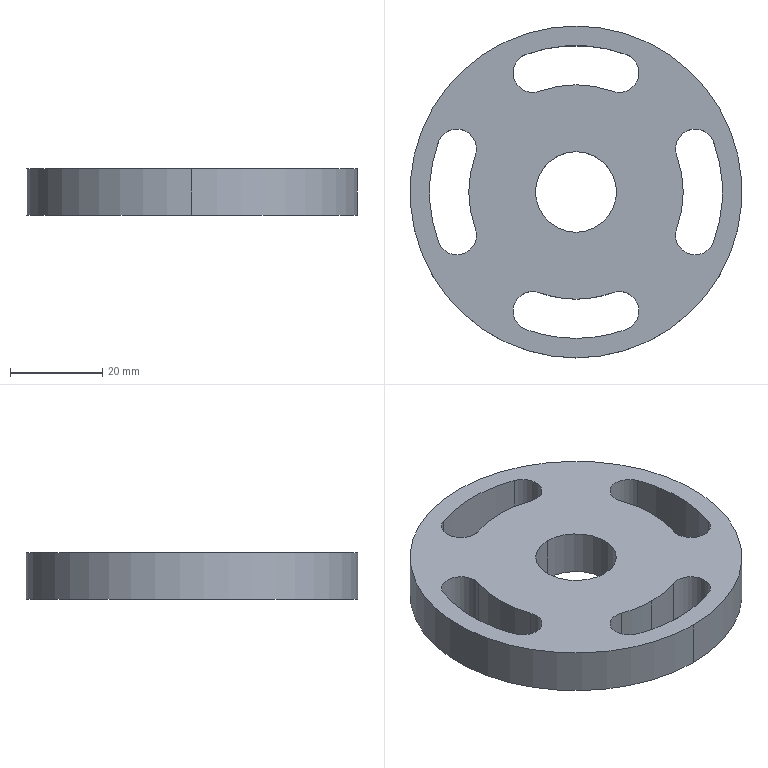Part | NX | 1 solid | 28 faces | box 72 x 72 x 10 mm | volume 29512 mm3 | cylinder 26 | plane 2 | commonest cylinder face diameters 8.5 x12 46.5 x5 63.5 x5 17.5 x2 72 x2
STEP:
#1=CARTESIAN_POINT('',(25.842,-13.656,0.));
#2=VERTEX_POINT('',#1);
#3=CARTESIAN_POINT('',(21.848,-7.952,0.));
#4=VERTEX_POINT('',#3);
#5=CARTESIAN_POINT('',(25.842,-9.406,0.));
#6=DIRECTION('',(0.,0.,-1.));
#7=DIRECTION('',(-1.,0.,0.));
#8=AXIS2_PLACEMENT_3D('',#5,#6,#7);
#9=CIRCLE('',#8,4.25);
#10=EDGE_CURVE('',#2,#4,#9,.T.);
#11=ORIENTED_EDGE('',*,*,#10,.F.);
#12=CARTESIAN_POINT('',(25.842,-13.656,-10.));
#13=VERTEX_POINT('',#12);
#14=CARTESIAN_POINT('',(25.842,-13.656,0.));
#15=DIRECTION('',(0.,0.,-1.));
#16=VECTOR('',#15,1000.);
#17=LINE('',#14,#16);
#18=EDGE_CURVE('',#2,#13,#17,.T.);
#19=ORIENTED_EDGE('',*,*,#18,.T.);
#20=CARTESIAN_POINT('',(21.848,-7.952,-10.));
#21=VERTEX_POINT('',#20);
#22=CARTESIAN_POINT('',(25.842,-9.406,-10.));
#23=DIRECTION('',(0.,0.,-1.));
#24=DIRECTION('',(-1.,0.,0.));
#25=AXIS2_PLACEMENT_3D('',#22,#23,#24);
#26=CIRCLE('',#25,4.25);
#27=EDGE_CURVE('',#13,#21,#26,.T.);
#28=ORIENTED_EDGE('',*,*,#27,.T.);
#29=CARTESIAN_POINT('',(21.848,-7.952,0.));
#30=DIRECTION('',(0.,0.,-1.));
#31=VECTOR('',#30,1000.);
#32=LINE('',#29,#31);
#33=EDGE_CURVE('',#4,#21,#32,.T.);
#34=ORIENTED_EDGE('',*,*,#33,.F.);
#35=EDGE_LOOP('',(#11,#19,#28,#34));
#36=FACE_BOUND('',#35,.T.);
#37=CARTESIAN_POINT('',(25.842,-9.406,0.));
#38=DIRECTION('',(0.,0.,-1.));
#39=DIRECTION('',(0.,1.,0.));
#40=AXIS2_PLACEMENT_3D('',#37,#38,#39);
#41=CYLINDRICAL_SURFACE('',#40,4.25);
#42=ADVANCED_FACE('',(#36),#41,.F.);
#43=CARTESIAN_POINT('',(0.,-31.75,0.));
#44=VERTEX_POINT('',#43);
#45=CARTESIAN_POINT('',(-10.859,-29.835,0.));
#46=VERTEX_POINT('',#45);
#47=CARTESIAN_POINT('',(0.,0.,0.));
#48=DIRECTION('',(0.,0.,-1.));
#49=DIRECTION('',(0.,1.,0.));
#50=AXIS2_PLACEMENT_3D('',#47,#48,#49);
#51=CIRCLE('',#50,31.75);
#52=EDGE_CURVE('',#44,#46,#51,.T.);
#53=ORIENTED_EDGE('',*,*,#52,.F.);
#54=CARTESIAN_POINT('',(0.,-31.75,-10.));
#55=VERTEX_POINT('',#54);
#56=CARTESIAN_POINT('',(0.,-31.75,0.));
#57=DIRECTION('',(0.,0.,-1.));
#58=VECTOR('',#57,1000.);
#59=LINE('',#56,#58);
#60=EDGE_CURVE('',#44,#55,#59,.T.);
#61=ORIENTED_EDGE('',*,*,#60,.T.);
#62=CARTESIAN_POINT('',(-10.859,-29.835,-10.));
#63=VERTEX_POINT('',#62);
#64=CARTESIAN_POINT('',(0.,0.,-10.));
#65=DIRECTION('',(0.,0.,-1.));
#66=DIRECTION('',(0.,1.,0.));
#67=AXIS2_PLACEMENT_3D('',#64,#65,#66);
#68=CIRCLE('',#67,31.75);
#69=EDGE_CURVE('',#55,#63,#68,.T.);
#70=ORIENTED_EDGE('',*,*,#69,.T.);
#71=CARTESIAN_POINT('',(-10.859,-29.835,0.));
#72=DIRECTION('',(0.,0.,-1.));
#73=VECTOR('',#72,1000.);
#74=LINE('',#71,#73);
#75=EDGE_CURVE('',#46,#63,#74,.T.);
#76=ORIENTED_EDGE('',*,*,#75,.F.);
#77=EDGE_LOOP('',(#53,#61,#70,#76));
#78=FACE_BOUND('',#77,.T.);
#79=CARTESIAN_POINT('',(0.,0.,0.));
#80=DIRECTION('',(0.,0.,-1.));
#81=DIRECTION('',(0.,1.,0.));
#82=AXIS2_PLACEMENT_3D('',#79,#80,#81);
#83=CYLINDRICAL_SURFACE('',#82,31.75);
#84=ADVANCED_FACE('',(#78),#83,.F.);
#85=CARTESIAN_POINT('',(0.,-23.25,0.));
#86=VERTEX_POINT('',#85);
#87=CARTESIAN_POINT('',(7.952,-21.848,0.));
#88=VERTEX_POINT('',#87);
#89=CARTESIAN_POINT('',(0.,0.,0.));
#90=DIRECTION('',(0.,0.,1.));
#91=DIRECTION('',(0.,1.,0.));
#92=AXIS2_PLACEMENT_3D('',#89,#90,#91);
#93=CIRCLE('',#92,23.25);
#94=EDGE_CURVE('',#86,#88,#93,.T.);
#95=ORIENTED_EDGE('',*,*,#94,.F.);
#96=CARTESIAN_POINT('',(0.,-23.25,-10.));
#97=VERTEX_POINT('',#96);
#98=CARTESIAN_POINT('',(0.,-23.25,0.));
#99=DIRECTION('',(0.,0.,-1.));
#100=VECTOR('',#99,1000.);
#101=LINE('',#98,#100);
#102=EDGE_CURVE('',#86,#97,#101,.T.);
#103=ORIENTED_EDGE('',*,*,#102,.T.);
#104=CARTESIAN_POINT('',(7.952,-21.848,-10.));
#105=VERTEX_POINT('',#104);
#106=CARTESIAN_POINT('',(0.,0.,-10.));
#107=DIRECTION('',(0.,0.,1.));
#108=DIRECTION('',(0.,1.,0.));
#109=AXIS2_PLACEMENT_3D('',#106,#107,#108);
#110=CIRCLE('',#109,23.25);
#111=EDGE_CURVE('',#97,#105,#110,.T.);
#112=ORIENTED_EDGE('',*,*,#111,.T.);
#113=CARTESIAN_POINT('',(7.952,-21.848,0.));
#114=DIRECTION('',(0.,0.,-1.));
#115=VECTOR('',#114,1000.);
#116=LINE('',#113,#115);
#117=EDGE_CURVE('',#88,#105,#116,.T.);
#118=ORIENTED_EDGE('',*,*,#117,.F.);
#119=EDGE_LOOP('',(#95,#103,#112,#118));
#120=FACE_BOUND('',#119,.T.);
#121=CARTESIAN_POINT('',(0.,0.,0.));
#122=DIRECTION('',(0.,0.,-1.));
#123=DIRECTION('',(0.,1.,0.));
#124=AXIS2_PLACEMENT_3D('',#121,#122,#123);
#125=CYLINDRICAL_SURFACE('',#124,23.25);
#126=ADVANCED_FACE('',(#120),#125,.T.);
#127=CARTESIAN_POINT('',(-25.842,-13.656,0.));
#128=VERTEX_POINT('',#127);
#129=CARTESIAN_POINT('',(-29.835,-10.859,0.));
#130=VERTEX_POINT('',#129);
#131=CARTESIAN_POINT('',(-25.842,-9.406,0.));
#132=DIRECTION('',(0.,0.,-1.));
#133=DIRECTION('',(1.,0.,0.));
#134=AXIS2_PLACEMENT_3D('',#131,#132,#133);
#135=CIRCLE('',#134,4.25);
#136=EDGE_CURVE('',#128,#130,#135,.T.);
#137=ORIENTED_EDGE('',*,*,#136,.F.);
#138=CARTESIAN_POINT('',(-25.842,-13.656,-10.));
#139=VERTEX_POINT('',#138);
#140=CARTESIAN_POINT('',(-25.842,-13.656,0.));
#141=DIRECTION('',(0.,0.,-1.));
#142=VECTOR('',#141,1000.);
#143=LINE('',#140,#142);
#144=EDGE_CURVE('',#128,#139,#143,.T.);
#145=ORIENTED_EDGE('',*,*,#144,.T.);
#146=CARTESIAN_POINT('',(-29.835,-10.859,-10.));
#147=VERTEX_POINT('',#146);
#148=CARTESIAN_POINT('',(-25.842,-9.406,-10.));
#149=DIRECTION('',(0.,0.,-1.));
#150=DIRECTION('',(1.,0.,0.));
#151=AXIS2_PLACEMENT_3D('',#148,#149,#150);
#152=CIRCLE('',#151,4.25);
#153=EDGE_CURVE('',#139,#147,#152,.T.);
#154=ORIENTED_EDGE('',*,*,#153,.T.);
#155=CARTESIAN_POINT('',(-29.835,-10.859,0.));
#156=DIRECTION('',(0.,0.,-1.));
#157=VECTOR('',#156,1000.);
#158=LINE('',#155,#157);
#159=EDGE_CURVE('',#130,#147,#158,.T.);
#160=ORIENTED_EDGE('',*,*,#159,.F.);
#161=EDGE_LOOP('',(#137,#145,#154,#160));
#162=FACE_BOUND('',#161,.T.);
#163=CARTESIAN_POINT('',(-25.842,-9.406,0.));
#164=DIRECTION('',(0.,0.,-1.));
#165=DIRECTION('',(0.,1.,0.));
#166=AXIS2_PLACEMENT_3D('',#163,#164,#165);
#167=CYLINDRICAL_SURFACE('',#166,4.25);
#168=ADVANCED_FACE('',(#162),#167,.F.);
#169=CARTESIAN_POINT('',(9.406,21.592,0.));
#170=VERTEX_POINT('',#169);
#171=CARTESIAN_POINT('',(7.952,21.848,0.));
#172=VERTEX_POINT('',#171);
#173=CARTESIAN_POINT('',(9.406,25.842,0.));
#174=DIRECTION('',(0.,0.,-1.));
#175=DIRECTION('',(0.,-1.,0.));
#176=AXIS2_PLACEMENT_3D('',#173,#174,#175);
#177=CIRCLE('',#176,4.25);
#178=EDGE_CURVE('',#170,#172,#177,.T.);
#179=ORIENTED_EDGE('',*,*,#178,.F.);
#180=CARTESIAN_POINT('',(9.406,21.592,-10.));
#181=VERTEX_POINT('',#180);
#182=CARTESIAN_POINT('',(9.406,21.592,0.));
#183=DIRECTION('',(0.,0.,-1.));
#184=VECTOR('',#183,1000.);
#185=LINE('',#182,#184);
#186=EDGE_CURVE('',#170,#181,#185,.T.);
#187=ORIENTED_EDGE('',*,*,#186,.T.);
#188=CARTESIAN_POINT('',(7.952,21.848,-10.));
#189=VERTEX_POINT('',#188);
#190=CARTESIAN_POINT('',(9.406,25.842,-10.));
#191=DIRECTION('',(0.,0.,-1.));
#192=DIRECTION('',(0.,-1.,0.));
#193=AXIS2_PLACEMENT_3D('',#190,#191,#192);
#194=CIRCLE('',#193,4.25);
#195=EDGE_CURVE('',#181,#189,#194,.T.);
#196=ORIENTED_EDGE('',*,*,#195,.T.);
#197=CARTESIAN_POINT('',(7.952,21.848,0.));
#198=DIRECTION('',(0.,0.,-1.));
#199=VECTOR('',#198,1000.);
#200=LINE('',#197,#199);
#201=EDGE_CURVE('',#172,#189,#200,.T.);
#202=ORIENTED_EDGE('',*,*,#201,.F.);
#203=EDGE_LOOP('',(#179,#187,#196,#202));
#204=FACE_BOUND('',#203,.T.);
#205=CARTESIAN_POINT('',(9.406,25.842,0.));
#206=DIRECTION('',(0.,0.,-1.));
#207=DIRECTION('',(0.,1.,0.));
#208=AXIS2_PLACEMENT_3D('',#205,#206,#207);
#209=CYLINDRICAL_SURFACE('',#208,4.25);
#210=ADVANCED_FACE('',(#204),#209,.F.);
#211=CARTESIAN_POINT('',(-9.406,21.592,0.));
#212=VERTEX_POINT('',#211);
#213=CARTESIAN_POINT('',(-10.859,29.835,0.));
#214=VERTEX_POINT('',#213);
#215=CARTESIAN_POINT('',(-9.406,25.842,0.));
#216=DIRECTION('',(0.,0.,-1.));
#217=DIRECTION('',(0.,-1.,0.));
#218=AXIS2_PLACEMENT_3D('',#215,#216,#217);
#219=CIRCLE('',#218,4.25);
#220=EDGE_CURVE('',#212,#214,#219,.T.);
#221=ORIENTED_EDGE('',*,*,#220,.F.);
#222=CARTESIAN_POINT('',(-9.406,21.592,-10.));
#223=VERTEX_POINT('',#222);
#224=CARTESIAN_POINT('',(-9.406,21.592,0.));
#225=DIRECTION('',(0.,0.,-1.));
#226=VECTOR('',#225,1000.);
#227=LINE('',#224,#226);
#228=EDGE_CURVE('',#212,#223,#227,.T.);
#229=ORIENTED_EDGE('',*,*,#228,.T.);
#230=CARTESIAN_POINT('',(-10.859,29.835,-10.));
#231=VERTEX_POINT('',#230);
#232=CARTESIAN_POINT('',(-9.406,25.842,-10.));
#233=DIRECTION('',(0.,0.,-1.));
#234=DIRECTION('',(0.,-1.,0.));
#235=AXIS2_PLACEMENT_3D('',#232,#233,#234);
#236=CIRCLE('',#235,4.25);
#237=EDGE_CURVE('',#223,#231,#236,.T.);
#238=ORIENTED_EDGE('',*,*,#237,.T.);
#239=CARTESIAN_POINT('',(-10.859,29.835,0.));
#240=DIRECTION('',(0.,0.,-1.));
#241=VECTOR('',#240,1000.);
#242=LINE('',#239,#241);
#243=EDGE_CURVE('',#214,#231,#242,.T.);
#244=ORIENTED_EDGE('',*,*,#243,.F.);
#245=EDGE_LOOP('',(#221,#229,#238,#244));
#246=FACE_BOUND('',#245,.T.);
#247=CARTESIAN_POINT('',(-9.406,25.842,0.));
#248=DIRECTION('',(0.,0.,-1.));
#249=DIRECTION('',(0.,1.,0.));
#250=AXIS2_PLACEMENT_3D('',#247,#248,#249);
#251=CYLINDRICAL_SURFACE('',#250,4.25);
#252=ADVANCED_FACE('',(#246),#251,.F.);
#253=CARTESIAN_POINT('',(0.,8.75,0.));
#254=VERTEX_POINT('',#253);
#255=CARTESIAN_POINT('',(0.,-8.75,0.));
#256=VERTEX_POINT('',#255);
#257=CARTESIAN_POINT('',(0.,0.,0.));
#258=DIRECTION('',(0.,0.,-1.));
#259=DIRECTION('',(0.,-1.,0.));
#260=AXIS2_PLACEMENT_3D('',#257,#258,#259);
#261=CIRCLE('',#260,8.75);
#262=EDGE_CURVE('',#254,#256,#261,.T.);
#263=ORIENTED_EDGE('',*,*,#262,.F.);
#264=CARTESIAN_POINT('',(0.,8.75,-10.));
#265=VERTEX_POINT('',#264);
#266=CARTESIAN_POINT('',(0.,8.75,-10.));
#267=DIRECTION('',(0.,0.,-1.));
#268=VECTOR('',#267,1000.);
#269=LINE('',#266,#268);
#270=EDGE_CURVE('',#265,#254,#269,.F.);
#271=ORIENTED_EDGE('',*,*,#270,.F.);
#272=CARTESIAN_POINT('',(0.,-8.75,-10.));
#273=VERTEX_POINT('',#272);
#274=CARTESIAN_POINT('',(0.,0.,-10.));
#275=DIRECTION('',(0.,0.,-1.));
#276=DIRECTION('',(0.,-1.,0.));
#277=AXIS2_PLACEMENT_3D('',#274,#275,#276);
#278=CIRCLE('',#277,8.75);
#279=EDGE_CURVE('',#265,#273,#278,.T.);
#280=ORIENTED_EDGE('',*,*,#279,.T.);
#281=CARTESIAN_POINT('',(0.,-8.75,-10.));
#282=DIRECTION('',(0.,0.,-1.));
#283=VECTOR('',#282,1000.);
#284=LINE('',#281,#283);
#285=EDGE_CURVE('',#273,#256,#284,.F.);
#286=ORIENTED_EDGE('',*,*,#285,.T.);
#287=EDGE_LOOP('',(#263,#271,#280,#286));
#288=FACE_BOUND('',#287,.T.);
#289=CARTESIAN_POINT('',(0.,0.,-10.));
#290=DIRECTION('',(0.,0.,-1.));
#291=DIRECTION('',(0.,1.,0.));
#292=AXIS2_PLACEMENT_3D('',#289,#290,#291);
#293=CYLINDRICAL_SURFACE('',#292,8.75);
#294=ADVANCED_FACE('',(#288),#293,.F.);
#295=CARTESIAN_POINT('',(0.,-36.,-10.));
#296=VERTEX_POINT('',#295);
#297=CARTESIAN_POINT('',(0.,36.,-10.));
#298=VERTEX_POINT('',#297);
#299=CARTESIAN_POINT('',(0.,0.,-10.));
#300=DIRECTION('',(0.,0.,-1.));
#301=DIRECTION('',(0.,-1.,0.));
#302=AXIS2_PLACEMENT_3D('',#299,#300,#301);
#303=CIRCLE('',#302,36.);
#304=EDGE_CURVE('',#296,#298,#303,.T.);
#305=ORIENTED_EDGE('',*,*,#304,.F.);
#306=CARTESIAN_POINT('',(0.,-36.,0.));
#307=VERTEX_POINT('',#306);
#308=CARTESIAN_POINT('',(0.,-36.,-10.));
#309=DIRECTION('',(0.,0.,1.));
#310=VECTOR('',#309,1000.);
#311=LINE('',#308,#310);
#312=EDGE_CURVE('',#307,#296,#311,.F.);
#313=ORIENTED_EDGE('',*,*,#312,.F.);
#314=CARTESIAN_POINT('',(0.,36.,0.));
#315=VERTEX_POINT('',#314);
#316=CARTESIAN_POINT('',(0.,0.,0.));
#317=DIRECTION('',(0.,0.,-1.));
#318=DIRECTION('',(0.,-1.,0.));
#319=AXIS2_PLACEMENT_3D('',#316,#317,#318);
#320=CIRCLE('',#319,36.);
#321=EDGE_CURVE('',#307,#315,#320,.T.);
#322=ORIENTED_EDGE('',*,*,#321,.T.);
#323=CARTESIAN_POINT('',(0.,36.,-10.));
#324=DIRECTION('',(0.,0.,1.));
#325=VECTOR('',#324,1000.);
#326=LINE('',#323,#325);
#327=EDGE_CURVE('',#315,#298,#326,.F.);
#328=ORIENTED_EDGE('',*,*,#327,.T.);
#329=EDGE_LOOP('',(#305,#313,#322,#328));
#330=FACE_BOUND('',#329,.T.);
#331=CARTESIAN_POINT('',(0.,0.,-10.));
#332=DIRECTION('',(0.,0.,1.));
#333=DIRECTION('',(0.,-1.,0.));
#334=AXIS2_PLACEMENT_3D('',#331,#332,#333);
#335=CYLINDRICAL_SURFACE('',#334,36.);
#336=ADVANCED_FACE('',(#330),#335,.T.);
#337=ORIENTED_EDGE('',*,*,#312,.T.);
#338=CARTESIAN_POINT('',(0.,0.,-10.));
#339=DIRECTION('',(0.,0.,-1.));
#340=DIRECTION('',(0.,-1.,0.));
#341=AXIS2_PLACEMENT_3D('',#338,#339,#340);
#342=CIRCLE('',#341,36.);
#343=EDGE_CURVE('',#298,#296,#342,.T.);
#344=ORIENTED_EDGE('',*,*,#343,.F.);
#345=ORIENTED_EDGE('',*,*,#327,.F.);
#346=CARTESIAN_POINT('',(0.,0.,0.));
#347=DIRECTION('',(0.,0.,-1.));
#348=DIRECTION('',(0.,-1.,0.));
#349=AXIS2_PLACEMENT_3D('',#346,#347,#348);
#350=CIRCLE('',#349,36.);
#351=EDGE_CURVE('',#315,#307,#350,.T.);
#352=ORIENTED_EDGE('',*,*,#351,.T.);
#353=EDGE_LOOP('',(#337,#344,#345,#352));
#354=FACE_BOUND('',#353,.T.);
#355=CARTESIAN_POINT('',(0.,0.,-10.));
#356=DIRECTION('',(0.,0.,1.));
#357=DIRECTION('',(0.,-1.,0.));
#358=AXIS2_PLACEMENT_3D('',#355,#356,#357);
#359=CYLINDRICAL_SURFACE('',#358,36.);
#360=ADVANCED_FACE('',(#354),#359,.T.);
#361=CARTESIAN_POINT('',(21.848,7.952,-10.));
#362=VERTEX_POINT('',#361);
#363=CARTESIAN_POINT('',(29.835,10.859,-10.));
#364=VERTEX_POINT('',#363);
#365=CARTESIAN_POINT('',(25.842,9.406,-10.));
#366=DIRECTION('',(0.,0.,-1.));
#367=DIRECTION('',(-1.,0.,0.));
#368=AXIS2_PLACEMENT_3D('',#365,#366,#367);
#369=CIRCLE('',#368,4.25);
#370=EDGE_CURVE('',#362,#364,#369,.T.);
#371=ORIENTED_EDGE('',*,*,#370,.F.);
#372=CARTESIAN_POINT('',(0.,0.,-10.));
#373=DIRECTION('',(0.,0.,1.));
#374=DIRECTION('',(-1.,0.,0.));
#375=AXIS2_PLACEMENT_3D('',#372,#373,#374);
#376=CIRCLE('',#375,23.25);
#377=EDGE_CURVE('',#21,#362,#376,.T.);
#378=ORIENTED_EDGE('',*,*,#377,.F.);
#379=ORIENTED_EDGE('',*,*,#27,.F.);
#380=CARTESIAN_POINT('',(29.835,-10.859,-10.));
#381=VERTEX_POINT('',#380);
#382=CARTESIAN_POINT('',(25.842,-9.406,-10.));
#383=DIRECTION('',(0.,0.,-1.));
#384=DIRECTION('',(-1.,0.,0.));
#385=AXIS2_PLACEMENT_3D('',#382,#383,#384);
#386=CIRCLE('',#385,4.25);
#387=EDGE_CURVE('',#381,#13,#386,.T.);
#388=ORIENTED_EDGE('',*,*,#387,.F.);
#389=CARTESIAN_POINT('',(0.,0.,-10.));
#390=DIRECTION('',(0.,0.,-1.));
#391=DIRECTION('',(-1.,0.,0.));
#392=AXIS2_PLACEMENT_3D('',#389,#390,#391);
#393=CIRCLE('',#392,31.75);
#394=EDGE_CURVE('',#364,#381,#393,.T.);
#395=ORIENTED_EDGE('',*,*,#394,.F.);
#396=EDGE_LOOP('',(#371,#378,#379,#388,#395));
#397=FACE_BOUND('',#396,.T.);
#398=CARTESIAN_POINT('',(10.859,-29.835,-10.));
#399=VERTEX_POINT('',#398);
#400=CARTESIAN_POINT('',(9.406,-25.842,-10.));
#401=DIRECTION('',(0.,0.,-1.));
#402=DIRECTION('',(0.,1.,0.));
#403=AXIS2_PLACEMENT_3D('',#400,#401,#402);
#404=CIRCLE('',#403,4.25);
#405=EDGE_CURVE('',#105,#399,#404,.T.);
#406=ORIENTED_EDGE('',*,*,#405,.F.);
#407=ORIENTED_EDGE('',*,*,#111,.F.);
#408=CARTESIAN_POINT('',(-7.952,-21.848,-10.));
#409=VERTEX_POINT('',#408);
#410=CARTESIAN_POINT('',(0.,0.,-10.));
#411=DIRECTION('',(0.,0.,1.));
#412=DIRECTION('',(0.,1.,0.));
#413=AXIS2_PLACEMENT_3D('',#410,#411,#412);
#414=CIRCLE('',#413,23.25);
#415=EDGE_CURVE('',#409,#97,#414,.T.);
#416=ORIENTED_EDGE('',*,*,#415,.F.);
#417=CARTESIAN_POINT('',(-9.406,-25.842,-10.));
#418=DIRECTION('',(0.,0.,-1.));
#419=DIRECTION('',(0.,1.,0.));
#420=AXIS2_PLACEMENT_3D('',#417,#418,#419);
#421=CIRCLE('',#420,4.25);
#422=EDGE_CURVE('',#63,#409,#421,.T.);
#423=ORIENTED_EDGE('',*,*,#422,.F.);
#424=ORIENTED_EDGE('',*,*,#69,.F.);
#425=CARTESIAN_POINT('',(0.,0.,-10.));
#426=DIRECTION('',(0.,0.,-1.));
#427=DIRECTION('',(0.,1.,0.));
#428=AXIS2_PLACEMENT_3D('',#425,#426,#427);
#429=CIRCLE('',#428,31.75);
#430=EDGE_CURVE('',#399,#55,#429,.T.);
#431=ORIENTED_EDGE('',*,*,#430,.F.);
#432=EDGE_LOOP('',(#406,#407,#416,#423,#424,#431));
#433=FACE_BOUND('',#432,.T.);
#434=CARTESIAN_POINT('',(-21.848,-7.952,-10.));
#435=VERTEX_POINT('',#434);
#436=CARTESIAN_POINT('',(-25.842,-9.406,-10.));
#437=DIRECTION('',(0.,0.,-1.));
#438=DIRECTION('',(1.,0.,0.));
#439=AXIS2_PLACEMENT_3D('',#436,#437,#438);
#440=CIRCLE('',#439,4.25);
#441=EDGE_CURVE('',#435,#139,#440,.T.);
#442=ORIENTED_EDGE('',*,*,#441,.F.);
#443=CARTESIAN_POINT('',(-21.848,7.952,-10.));
#444=VERTEX_POINT('',#443);
#445=CARTESIAN_POINT('',(0.,0.,-10.));
#446=DIRECTION('',(0.,0.,1.));
#447=DIRECTION('',(1.,0.,0.));
#448=AXIS2_PLACEMENT_3D('',#445,#446,#447);
#449=CIRCLE('',#448,23.25);
#450=EDGE_CURVE('',#444,#435,#449,.T.);
#451=ORIENTED_EDGE('',*,*,#450,.F.);
#452=CARTESIAN_POINT('',(-29.835,10.859,-10.));
#453=VERTEX_POINT('',#452);
#454=CARTESIAN_POINT('',(-25.842,9.406,-10.));
#455=DIRECTION('',(0.,0.,-1.));
#456=DIRECTION('',(1.,0.,0.));
#457=AXIS2_PLACEMENT_3D('',#454,#455,#456);
#458=CIRCLE('',#457,4.25);
#459=EDGE_CURVE('',#453,#444,#458,.T.);
#460=ORIENTED_EDGE('',*,*,#459,.F.);
#461=CARTESIAN_POINT('',(0.,0.,-10.));
#462=DIRECTION('',(0.,0.,-1.));
#463=DIRECTION('',(1.,0.,0.));
#464=AXIS2_PLACEMENT_3D('',#461,#462,#463);
#465=CIRCLE('',#464,31.75);
#466=EDGE_CURVE('',#147,#453,#465,.T.);
#467=ORIENTED_EDGE('',*,*,#466,.F.);
#468=ORIENTED_EDGE('',*,*,#153,.F.);
#469=EDGE_LOOP('',(#442,#451,#460,#467,#468));
#470=FACE_BOUND('',#469,.T.);
#471=CARTESIAN_POINT('',(-7.952,21.848,-10.));
#472=VERTEX_POINT('',#471);
#473=CARTESIAN_POINT('',(-9.406,25.842,-10.));
#474=DIRECTION('',(0.,0.,-1.));
#475=DIRECTION('',(0.,-1.,0.));
#476=AXIS2_PLACEMENT_3D('',#473,#474,#475);
#477=CIRCLE('',#476,4.25);
#478=EDGE_CURVE('',#472,#223,#477,.T.);
#479=ORIENTED_EDGE('',*,*,#478,.F.);
#480=CARTESIAN_POINT('',(0.,0.,-10.));
#481=DIRECTION('',(0.,0.,1.));
#482=DIRECTION('',(0.,-1.,0.));
#483=AXIS2_PLACEMENT_3D('',#480,#481,#482);
#484=CIRCLE('',#483,23.25);
#485=EDGE_CURVE('',#189,#472,#484,.T.);
#486=ORIENTED_EDGE('',*,*,#485,.F.);
#487=ORIENTED_EDGE('',*,*,#195,.F.);
#488=CARTESIAN_POINT('',(10.859,29.835,-10.));
#489=VERTEX_POINT('',#488);
#490=CARTESIAN_POINT('',(9.406,25.842,-10.));
#491=DIRECTION('',(0.,0.,-1.));
#492=DIRECTION('',(0.,-1.,0.));
#493=AXIS2_PLACEMENT_3D('',#490,#491,#492);
#494=CIRCLE('',#493,4.25);
#495=EDGE_CURVE('',#489,#181,#494,.T.);
#496=ORIENTED_EDGE('',*,*,#495,.F.);
#497=CARTESIAN_POINT('',(0.,0.,-10.));
#498=DIRECTION('',(0.,0.,-1.));
#499=DIRECTION('',(0.,-1.,0.));
#500=AXIS2_PLACEMENT_3D('',#497,#498,#499);
#501=CIRCLE('',#500,31.75);
#502=EDGE_CURVE('',#231,#489,#501,.T.);
#503=ORIENTED_EDGE('',*,*,#502,.F.);
#504=ORIENTED_EDGE('',*,*,#237,.F.);
#505=EDGE_LOOP('',(#479,#486,#487,#496,#503,#504));
#506=FACE_BOUND('',#505,.T.);
#507=CARTESIAN_POINT('',(0.,0.,-10.));
#508=DIRECTION('',(0.,0.,-1.));
#509=DIRECTION('',(0.,-1.,0.));
#510=AXIS2_PLACEMENT_3D('',#507,#508,#509);
#511=CIRCLE('',#510,8.75);
#512=EDGE_CURVE('',#273,#265,#511,.T.);
#513=ORIENTED_EDGE('',*,*,#512,.F.);
#514=ORIENTED_EDGE('',*,*,#279,.F.);
#515=EDGE_LOOP('',(#513,#514));
#516=FACE_BOUND('',#515,.T.);
#517=ORIENTED_EDGE('',*,*,#343,.T.);
#518=ORIENTED_EDGE('',*,*,#304,.T.);
#519=EDGE_LOOP('',(#517,#518));
#520=FACE_BOUND('',#519,.T.);
#521=CARTESIAN_POINT('',(0.,0.,-10.));
#522=DIRECTION('',(0.,0.,-1.));
#523=DIRECTION('',(0.,1.,0.));
#524=AXIS2_PLACEMENT_3D('',#521,#522,#523);
#525=PLANE('',#524);
#526=ADVANCED_FACE('',(#397,#433,#470,#506,#516,#520),#525,.T.);
#527=CARTESIAN_POINT('',(21.848,7.952,0.));
#528=VERTEX_POINT('',#527);
#529=CARTESIAN_POINT('',(0.,0.,0.));
#530=DIRECTION('',(0.,0.,1.));
#531=DIRECTION('',(-1.,0.,0.));
#532=AXIS2_PLACEMENT_3D('',#529,#530,#531);
#533=CIRCLE('',#532,23.25);
#534=EDGE_CURVE('',#4,#528,#533,.T.);
#535=ORIENTED_EDGE('',*,*,#534,.T.);
#536=CARTESIAN_POINT('',(29.835,10.859,0.));
#537=VERTEX_POINT('',#536);
#538=CARTESIAN_POINT('',(25.842,9.406,0.));
#539=DIRECTION('',(0.,0.,-1.));
#540=DIRECTION('',(-1.,0.,0.));
#541=AXIS2_PLACEMENT_3D('',#538,#539,#540);
#542=CIRCLE('',#541,4.25);
#543=EDGE_CURVE('',#528,#537,#542,.T.);
#544=ORIENTED_EDGE('',*,*,#543,.T.);
#545=CARTESIAN_POINT('',(29.835,-10.859,0.));
#546=VERTEX_POINT('',#545);
#547=CARTESIAN_POINT('',(0.,0.,0.));
#548=DIRECTION('',(0.,0.,-1.));
#549=DIRECTION('',(-1.,0.,0.));
#550=AXIS2_PLACEMENT_3D('',#547,#548,#549);
#551=CIRCLE('',#550,31.75);
#552=EDGE_CURVE('',#537,#546,#551,.T.);
#553=ORIENTED_EDGE('',*,*,#552,.T.);
#554=CARTESIAN_POINT('',(25.842,-9.406,0.));
#555=DIRECTION('',(0.,0.,-1.));
#556=DIRECTION('',(-1.,0.,0.));
#557=AXIS2_PLACEMENT_3D('',#554,#555,#556);
#558=CIRCLE('',#557,4.25);
#559=EDGE_CURVE('',#546,#2,#558,.T.);
#560=ORIENTED_EDGE('',*,*,#559,.T.);
#561=ORIENTED_EDGE('',*,*,#10,.T.);
#562=EDGE_LOOP('',(#535,#544,#553,#560,#561));
#563=FACE_BOUND('',#562,.T.);
#564=CARTESIAN_POINT('',(-7.952,-21.848,0.));
#565=VERTEX_POINT('',#564);
#566=CARTESIAN_POINT('',(0.,0.,0.));
#567=DIRECTION('',(0.,0.,1.));
#568=DIRECTION('',(0.,1.,0.));
#569=AXIS2_PLACEMENT_3D('',#566,#567,#568);
#570=CIRCLE('',#569,23.25);
#571=EDGE_CURVE('',#565,#86,#570,.T.);
#572=ORIENTED_EDGE('',*,*,#571,.T.);
#573=ORIENTED_EDGE('',*,*,#94,.T.);
#574=CARTESIAN_POINT('',(10.859,-29.835,0.));
#575=VERTEX_POINT('',#574);
#576=CARTESIAN_POINT('',(9.406,-25.842,0.));
#577=DIRECTION('',(0.,0.,-1.));
#578=DIRECTION('',(0.,1.,0.));
#579=AXIS2_PLACEMENT_3D('',#576,#577,#578);
#580=CIRCLE('',#579,4.25);
#581=EDGE_CURVE('',#88,#575,#580,.T.);
#582=ORIENTED_EDGE('',*,*,#581,.T.);
#583=CARTESIAN_POINT('',(0.,0.,0.));
#584=DIRECTION('',(0.,0.,-1.));
#585=DIRECTION('',(0.,1.,0.));
#586=AXIS2_PLACEMENT_3D('',#583,#584,#585);
#587=CIRCLE('',#586,31.75);
#588=EDGE_CURVE('',#575,#44,#587,.T.);
#589=ORIENTED_EDGE('',*,*,#588,.T.);
#590=ORIENTED_EDGE('',*,*,#52,.T.);
#591=CARTESIAN_POINT('',(-9.406,-25.842,0.));
#592=DIRECTION('',(0.,0.,-1.));
#593=DIRECTION('',(0.,1.,0.));
#594=AXIS2_PLACEMENT_3D('',#591,#592,#593);
#595=CIRCLE('',#594,4.25);
#596=EDGE_CURVE('',#46,#565,#595,.T.);
#597=ORIENTED_EDGE('',*,*,#596,.T.);
#598=EDGE_LOOP('',(#572,#573,#582,#589,#590,#597));
#599=FACE_BOUND('',#598,.T.);
#600=CARTESIAN_POINT('',(-21.848,7.952,0.));
#601=VERTEX_POINT('',#600);
#602=CARTESIAN_POINT('',(-21.848,-7.952,0.));
#603=VERTEX_POINT('',#602);
#604=CARTESIAN_POINT('',(0.,0.,0.));
#605=DIRECTION('',(0.,0.,1.));
#606=DIRECTION('',(1.,0.,0.));
#607=AXIS2_PLACEMENT_3D('',#604,#605,#606);
#608=CIRCLE('',#607,23.25);
#609=EDGE_CURVE('',#601,#603,#608,.T.);
#610=ORIENTED_EDGE('',*,*,#609,.T.);
#611=CARTESIAN_POINT('',(-25.842,-9.406,0.));
#612=DIRECTION('',(0.,0.,-1.));
#613=DIRECTION('',(1.,0.,0.));
#614=AXIS2_PLACEMENT_3D('',#611,#612,#613);
#615=CIRCLE('',#614,4.25);
#616=EDGE_CURVE('',#603,#128,#615,.T.);
#617=ORIENTED_EDGE('',*,*,#616,.T.);
#618=ORIENTED_EDGE('',*,*,#136,.T.);
#619=CARTESIAN_POINT('',(-29.835,10.859,0.));
#620=VERTEX_POINT('',#619);
#621=CARTESIAN_POINT('',(0.,0.,0.));
#622=DIRECTION('',(0.,0.,-1.));
#623=DIRECTION('',(1.,0.,0.));
#624=AXIS2_PLACEMENT_3D('',#621,#622,#623);
#625=CIRCLE('',#624,31.75);
#626=EDGE_CURVE('',#130,#620,#625,.T.);
#627=ORIENTED_EDGE('',*,*,#626,.T.);
#628=CARTESIAN_POINT('',(-25.842,9.406,0.));
#629=DIRECTION('',(0.,0.,-1.));
#630=DIRECTION('',(1.,0.,0.));
#631=AXIS2_PLACEMENT_3D('',#628,#629,#630);
#632=CIRCLE('',#631,4.25);
#633=EDGE_CURVE('',#620,#601,#632,.T.);
#634=ORIENTED_EDGE('',*,*,#633,.T.);
#635=EDGE_LOOP('',(#610,#617,#618,#627,#634));
#636=FACE_BOUND('',#635,.T.);
#637=CARTESIAN_POINT('',(-7.952,21.848,0.));
#638=VERTEX_POINT('',#637);
#639=CARTESIAN_POINT('',(0.,0.,0.));
#640=DIRECTION('',(0.,0.,1.));
#641=DIRECTION('',(0.,-1.,0.));
#642=AXIS2_PLACEMENT_3D('',#639,#640,#641);
#643=CIRCLE('',#642,23.25);
#644=EDGE_CURVE('',#172,#638,#643,.T.);
#645=ORIENTED_EDGE('',*,*,#644,.T.);
#646=CARTESIAN_POINT('',(-9.406,25.842,0.));
#647=DIRECTION('',(0.,0.,-1.));
#648=DIRECTION('',(0.,-1.,0.));
#649=AXIS2_PLACEMENT_3D('',#646,#647,#648);
#650=CIRCLE('',#649,4.25);
#651=EDGE_CURVE('',#638,#212,#650,.T.);
#652=ORIENTED_EDGE('',*,*,#651,.T.);
#653=ORIENTED_EDGE('',*,*,#220,.T.);
#654=CARTESIAN_POINT('',(10.859,29.835,0.));
#655=VERTEX_POINT('',#654);
#656=CARTESIAN_POINT('',(0.,0.,0.));
#657=DIRECTION('',(0.,0.,-1.));
#658=DIRECTION('',(0.,-1.,0.));
#659=AXIS2_PLACEMENT_3D('',#656,#657,#658);
#660=CIRCLE('',#659,31.75);
#661=EDGE_CURVE('',#214,#655,#660,.T.);
#662=ORIENTED_EDGE('',*,*,#661,.T.);
#663=CARTESIAN_POINT('',(9.406,25.842,0.));
#664=DIRECTION('',(0.,0.,-1.));
#665=DIRECTION('',(0.,-1.,0.));
#666=AXIS2_PLACEMENT_3D('',#663,#664,#665);
#667=CIRCLE('',#666,4.25);
#668=EDGE_CURVE('',#655,#170,#667,.T.);
#669=ORIENTED_EDGE('',*,*,#668,.T.);
#670=ORIENTED_EDGE('',*,*,#178,.T.);
#671=EDGE_LOOP('',(#645,#652,#653,#662,#669,#670));
#672=FACE_BOUND('',#671,.T.);
#673=CARTESIAN_POINT('',(0.,0.,0.));
#674=DIRECTION('',(0.,0.,-1.));
#675=DIRECTION('',(0.,-1.,0.));
#676=AXIS2_PLACEMENT_3D('',#673,#674,#675);
#677=CIRCLE('',#676,8.75);
#678=EDGE_CURVE('',#256,#254,#677,.T.);
#679=ORIENTED_EDGE('',*,*,#678,.T.);
#680=ORIENTED_EDGE('',*,*,#262,.T.);
#681=EDGE_LOOP('',(#679,#680));
#682=FACE_BOUND('',#681,.T.);
#683=ORIENTED_EDGE('',*,*,#351,.F.);
#684=ORIENTED_EDGE('',*,*,#321,.F.);
#685=EDGE_LOOP('',(#683,#684));
#686=FACE_BOUND('',#685,.T.);
#687=CARTESIAN_POINT('',(0.,0.,0.));
#688=DIRECTION('',(0.,0.,-1.));
#689=DIRECTION('',(0.,1.,0.));
#690=AXIS2_PLACEMENT_3D('',#687,#688,#689);
#691=PLANE('',#690);
#692=ADVANCED_FACE('',(#563,#599,#636,#672,#682,#686),#691,.F.);
#693=ORIENTED_EDGE('',*,*,#270,.T.);
#694=ORIENTED_EDGE('',*,*,#678,.F.);
#695=ORIENTED_EDGE('',*,*,#285,.F.);
#696=ORIENTED_EDGE('',*,*,#512,.T.);
#697=EDGE_LOOP('',(#693,#694,#695,#696));
#698=FACE_BOUND('',#697,.T.);
#699=CARTESIAN_POINT('',(0.,0.,-10.));
#700=DIRECTION('',(0.,0.,-1.));
#701=DIRECTION('',(0.,1.,0.));
#702=AXIS2_PLACEMENT_3D('',#699,#700,#701);
#703=CYLINDRICAL_SURFACE('',#702,8.75);
#704=ADVANCED_FACE('',(#698),#703,.F.);
#705=ORIENTED_EDGE('',*,*,#228,.F.);
#706=ORIENTED_EDGE('',*,*,#651,.F.);
#707=CARTESIAN_POINT('',(-7.952,21.848,0.));
#708=DIRECTION('',(0.,0.,-1.));
#709=VECTOR('',#708,1000.);
#710=LINE('',#707,#709);
#711=EDGE_CURVE('',#638,#472,#710,.T.);
#712=ORIENTED_EDGE('',*,*,#711,.T.);
#713=ORIENTED_EDGE('',*,*,#478,.T.);
#714=EDGE_LOOP('',(#705,#706,#712,#713));
#715=FACE_BOUND('',#714,.T.);
#716=CARTESIAN_POINT('',(-9.406,25.842,0.));
#717=DIRECTION('',(0.,0.,-1.));
#718=DIRECTION('',(0.,1.,0.));
#719=AXIS2_PLACEMENT_3D('',#716,#717,#718);
#720=CYLINDRICAL_SURFACE('',#719,4.25);
#721=ADVANCED_FACE('',(#715),#720,.F.);
#722=ORIENTED_EDGE('',*,*,#485,.T.);
#723=ORIENTED_EDGE('',*,*,#711,.F.);
#724=ORIENTED_EDGE('',*,*,#644,.F.);
#725=ORIENTED_EDGE('',*,*,#201,.T.);
#726=EDGE_LOOP('',(#722,#723,#724,#725));
#727=FACE_BOUND('',#726,.T.);
#728=CARTESIAN_POINT('',(0.,0.,0.));
#729=DIRECTION('',(0.,0.,-1.));
#730=DIRECTION('',(0.,1.,0.));
#731=AXIS2_PLACEMENT_3D('',#728,#729,#730);
#732=CYLINDRICAL_SURFACE('',#731,23.25);
#733=ADVANCED_FACE('',(#727),#732,.T.);
#734=ORIENTED_EDGE('',*,*,#186,.F.);
#735=ORIENTED_EDGE('',*,*,#668,.F.);
#736=CARTESIAN_POINT('',(10.859,29.835,0.));
#737=DIRECTION('',(0.,0.,-1.));
#738=VECTOR('',#737,1000.);
#739=LINE('',#736,#738);
#740=EDGE_CURVE('',#655,#489,#739,.T.);
#741=ORIENTED_EDGE('',*,*,#740,.T.);
#742=ORIENTED_EDGE('',*,*,#495,.T.);
#743=EDGE_LOOP('',(#734,#735,#741,#742));
#744=FACE_BOUND('',#743,.T.);
#745=CARTESIAN_POINT('',(9.406,25.842,0.));
#746=DIRECTION('',(0.,0.,-1.));
#747=DIRECTION('',(0.,1.,0.));
#748=AXIS2_PLACEMENT_3D('',#745,#746,#747);
#749=CYLINDRICAL_SURFACE('',#748,4.25);
#750=ADVANCED_FACE('',(#744),#749,.F.);
#751=ORIENTED_EDGE('',*,*,#502,.T.);
#752=ORIENTED_EDGE('',*,*,#740,.F.);
#753=ORIENTED_EDGE('',*,*,#661,.F.);
#754=ORIENTED_EDGE('',*,*,#243,.T.);
#755=EDGE_LOOP('',(#751,#752,#753,#754));
#756=FACE_BOUND('',#755,.T.);
#757=CARTESIAN_POINT('',(0.,0.,0.));
#758=DIRECTION('',(0.,0.,-1.));
#759=DIRECTION('',(0.,1.,0.));
#760=AXIS2_PLACEMENT_3D('',#757,#758,#759);
#761=CYLINDRICAL_SURFACE('',#760,31.75);
#762=ADVANCED_FACE('',(#756),#761,.F.);
#763=ORIENTED_EDGE('',*,*,#144,.F.);
#764=ORIENTED_EDGE('',*,*,#616,.F.);
#765=CARTESIAN_POINT('',(-21.848,-7.952,0.));
#766=DIRECTION('',(0.,0.,-1.));
#767=VECTOR('',#766,1000.);
#768=LINE('',#765,#767);
#769=EDGE_CURVE('',#603,#435,#768,.T.);
#770=ORIENTED_EDGE('',*,*,#769,.T.);
#771=ORIENTED_EDGE('',*,*,#441,.T.);
#772=EDGE_LOOP('',(#763,#764,#770,#771));
#773=FACE_BOUND('',#772,.T.);
#774=CARTESIAN_POINT('',(-25.842,-9.406,0.));
#775=DIRECTION('',(0.,0.,-1.));
#776=DIRECTION('',(0.,1.,0.));
#777=AXIS2_PLACEMENT_3D('',#774,#775,#776);
#778=CYLINDRICAL_SURFACE('',#777,4.25);
#779=ADVANCED_FACE('',(#773),#778,.F.);
#780=ORIENTED_EDGE('',*,*,#450,.T.);
#781=ORIENTED_EDGE('',*,*,#769,.F.);
#782=ORIENTED_EDGE('',*,*,#609,.F.);
#783=CARTESIAN_POINT('',(-21.848,7.952,0.));
#784=DIRECTION('',(0.,0.,-1.));
#785=VECTOR('',#784,1000.);
#786=LINE('',#783,#785);
#787=EDGE_CURVE('',#601,#444,#786,.T.);
#788=ORIENTED_EDGE('',*,*,#787,.T.);
#789=EDGE_LOOP('',(#780,#781,#782,#788));
#790=FACE_BOUND('',#789,.T.);
#791=CARTESIAN_POINT('',(0.,0.,0.));
#792=DIRECTION('',(0.,0.,-1.));
#793=DIRECTION('',(0.,1.,0.));
#794=AXIS2_PLACEMENT_3D('',#791,#792,#793);
#795=CYLINDRICAL_SURFACE('',#794,23.25);
#796=ADVANCED_FACE('',(#790),#795,.T.);
#797=ORIENTED_EDGE('',*,*,#459,.T.);
#798=ORIENTED_EDGE('',*,*,#787,.F.);
#799=ORIENTED_EDGE('',*,*,#633,.F.);
#800=CARTESIAN_POINT('',(-29.835,10.859,0.));
#801=DIRECTION('',(0.,0.,-1.));
#802=VECTOR('',#801,1000.);
#803=LINE('',#800,#802);
#804=EDGE_CURVE('',#620,#453,#803,.T.);
#805=ORIENTED_EDGE('',*,*,#804,.T.);
#806=EDGE_LOOP('',(#797,#798,#799,#805));
#807=FACE_BOUND('',#806,.T.);
#808=CARTESIAN_POINT('',(-25.842,9.406,0.));
#809=DIRECTION('',(0.,0.,-1.));
#810=DIRECTION('',(0.,1.,0.));
#811=AXIS2_PLACEMENT_3D('',#808,#809,#810);
#812=CYLINDRICAL_SURFACE('',#811,4.25);
#813=ADVANCED_FACE('',(#807),#812,.F.);
#814=ORIENTED_EDGE('',*,*,#466,.T.);
#815=ORIENTED_EDGE('',*,*,#804,.F.);
#816=ORIENTED_EDGE('',*,*,#626,.F.);
#817=ORIENTED_EDGE('',*,*,#159,.T.);
#818=EDGE_LOOP('',(#814,#815,#816,#817));
#819=FACE_BOUND('',#818,.T.);
#820=CARTESIAN_POINT('',(0.,0.,0.));
#821=DIRECTION('',(0.,0.,-1.));
#822=DIRECTION('',(0.,1.,0.));
#823=AXIS2_PLACEMENT_3D('',#820,#821,#822);
#824=CYLINDRICAL_SURFACE('',#823,31.75);
#825=ADVANCED_FACE('',(#819),#824,.F.);
#826=ORIENTED_EDGE('',*,*,#405,.T.);
#827=CARTESIAN_POINT('',(10.859,-29.835,0.));
#828=DIRECTION('',(0.,0.,-1.));
#829=VECTOR('',#828,1000.);
#830=LINE('',#827,#829);
#831=EDGE_CURVE('',#575,#399,#830,.T.);
#832=ORIENTED_EDGE('',*,*,#831,.F.);
#833=ORIENTED_EDGE('',*,*,#581,.F.);
#834=ORIENTED_EDGE('',*,*,#117,.T.);
#835=EDGE_LOOP('',(#826,#832,#833,#834));
#836=FACE_BOUND('',#835,.T.);
#837=CARTESIAN_POINT('',(9.406,-25.842,0.));
#838=DIRECTION('',(0.,0.,-1.));
#839=DIRECTION('',(0.,1.,0.));
#840=AXIS2_PLACEMENT_3D('',#837,#838,#839);
#841=CYLINDRICAL_SURFACE('',#840,4.25);
#842=ADVANCED_FACE('',(#836),#841,.F.);
#843=ORIENTED_EDGE('',*,*,#102,.F.);
#844=ORIENTED_EDGE('',*,*,#571,.F.);
#845=CARTESIAN_POINT('',(-7.952,-21.848,0.));
#846=DIRECTION('',(0.,0.,-1.));
#847=VECTOR('',#846,1000.);
#848=LINE('',#845,#847);
#849=EDGE_CURVE('',#565,#409,#848,.T.);
#850=ORIENTED_EDGE('',*,*,#849,.T.);
#851=ORIENTED_EDGE('',*,*,#415,.T.);
#852=EDGE_LOOP('',(#843,#844,#850,#851));
#853=FACE_BOUND('',#852,.T.);
#854=CARTESIAN_POINT('',(0.,0.,0.));
#855=DIRECTION('',(0.,0.,-1.));
#856=DIRECTION('',(0.,1.,0.));
#857=AXIS2_PLACEMENT_3D('',#854,#855,#856);
#858=CYLINDRICAL_SURFACE('',#857,23.25);
#859=ADVANCED_FACE('',(#853),#858,.T.);
#860=ORIENTED_EDGE('',*,*,#422,.T.);
#861=ORIENTED_EDGE('',*,*,#849,.F.);
#862=ORIENTED_EDGE('',*,*,#596,.F.);
#863=ORIENTED_EDGE('',*,*,#75,.T.);
#864=EDGE_LOOP('',(#860,#861,#862,#863));
#865=FACE_BOUND('',#864,.T.);
#866=CARTESIAN_POINT('',(-9.406,-25.842,0.));
#867=DIRECTION('',(0.,0.,-1.));
#868=DIRECTION('',(0.,1.,0.));
#869=AXIS2_PLACEMENT_3D('',#866,#867,#868);
#870=CYLINDRICAL_SURFACE('',#869,4.25);
#871=ADVANCED_FACE('',(#865),#870,.F.);
#872=ORIENTED_EDGE('',*,*,#60,.F.);
#873=ORIENTED_EDGE('',*,*,#588,.F.);
#874=ORIENTED_EDGE('',*,*,#831,.T.);
#875=ORIENTED_EDGE('',*,*,#430,.T.);
#876=EDGE_LOOP('',(#872,#873,#874,#875));
#877=FACE_BOUND('',#876,.T.);
#878=CARTESIAN_POINT('',(0.,0.,0.));
#879=DIRECTION('',(0.,0.,-1.));
#880=DIRECTION('',(0.,1.,0.));
#881=AXIS2_PLACEMENT_3D('',#878,#879,#880);
#882=CYLINDRICAL_SURFACE('',#881,31.75);
#883=ADVANCED_FACE('',(#877),#882,.F.);
#884=ORIENTED_EDGE('',*,*,#370,.T.);
#885=CARTESIAN_POINT('',(29.835,10.859,0.));
#886=DIRECTION('',(0.,0.,-1.));
#887=VECTOR('',#886,1000.);
#888=LINE('',#885,#887);
#889=EDGE_CURVE('',#537,#364,#888,.T.);
#890=ORIENTED_EDGE('',*,*,#889,.F.);
#891=ORIENTED_EDGE('',*,*,#543,.F.);
#892=CARTESIAN_POINT('',(21.848,7.952,0.));
#893=DIRECTION('',(0.,0.,-1.));
#894=VECTOR('',#893,1000.);
#895=LINE('',#892,#894);
#896=EDGE_CURVE('',#528,#362,#895,.T.);
#897=ORIENTED_EDGE('',*,*,#896,.T.);
#898=EDGE_LOOP('',(#884,#890,#891,#897));
#899=FACE_BOUND('',#898,.T.);
#900=CARTESIAN_POINT('',(25.842,9.406,0.));
#901=DIRECTION('',(0.,0.,-1.));
#902=DIRECTION('',(0.,1.,0.));
#903=AXIS2_PLACEMENT_3D('',#900,#901,#902);
#904=CYLINDRICAL_SURFACE('',#903,4.25);
#905=ADVANCED_FACE('',(#899),#904,.F.);
#906=ORIENTED_EDGE('',*,*,#377,.T.);
#907=ORIENTED_EDGE('',*,*,#896,.F.);
#908=ORIENTED_EDGE('',*,*,#534,.F.);
#909=ORIENTED_EDGE('',*,*,#33,.T.);
#910=EDGE_LOOP('',(#906,#907,#908,#909));
#911=FACE_BOUND('',#910,.T.);
#912=CARTESIAN_POINT('',(0.,0.,0.));
#913=DIRECTION('',(0.,0.,-1.));
#914=DIRECTION('',(0.,1.,0.));
#915=AXIS2_PLACEMENT_3D('',#912,#913,#914);
#916=CYLINDRICAL_SURFACE('',#915,23.25);
#917=ADVANCED_FACE('',(#911),#916,.T.);
#918=ORIENTED_EDGE('',*,*,#18,.F.);
#919=ORIENTED_EDGE('',*,*,#559,.F.);
#920=CARTESIAN_POINT('',(29.835,-10.859,0.));
#921=DIRECTION('',(0.,0.,-1.));
#922=VECTOR('',#921,1000.);
#923=LINE('',#920,#922);
#924=EDGE_CURVE('',#546,#381,#923,.T.);
#925=ORIENTED_EDGE('',*,*,#924,.T.);
#926=ORIENTED_EDGE('',*,*,#387,.T.);
#927=EDGE_LOOP('',(#918,#919,#925,#926));
#928=FACE_BOUND('',#927,.T.);
#929=CARTESIAN_POINT('',(25.842,-9.406,0.));
#930=DIRECTION('',(0.,0.,-1.));
#931=DIRECTION('',(0.,1.,0.));
#932=AXIS2_PLACEMENT_3D('',#929,#930,#931);
#933=CYLINDRICAL_SURFACE('',#932,4.25);
#934=ADVANCED_FACE('',(#928),#933,.F.);
#935=ORIENTED_EDGE('',*,*,#394,.T.);
#936=ORIENTED_EDGE('',*,*,#924,.F.);
#937=ORIENTED_EDGE('',*,*,#552,.F.);
#938=ORIENTED_EDGE('',*,*,#889,.T.);
#939=EDGE_LOOP('',(#935,#936,#937,#938));
#940=FACE_BOUND('',#939,.T.);
#941=CARTESIAN_POINT('',(0.,0.,0.));
#942=DIRECTION('',(0.,0.,-1.));
#943=DIRECTION('',(0.,1.,0.));
#944=AXIS2_PLACEMENT_3D('',#941,#942,#943);
#945=CYLINDRICAL_SURFACE('',#944,31.75);
#946=ADVANCED_FACE('',(#940),#945,.F.);
#947=CLOSED_SHELL('',(#42,#84,#126,#168,#210,#252,#294,#336,#360,#526,#692,#704,#721,#733,#750,#762,#779,#796,#813,#825,#842,#859,#871,#883,#905,#917,#934,#946));
#948=MANIFOLD_SOLID_BREP('',#947);
#949=(LENGTH_UNIT()NAMED_UNIT(*)SI_UNIT(.MILLI.,.METRE.));
#950=UNCERTAINTY_MEASURE_WITH_UNIT(LENGTH_MEASURE(0.00001),#949,'','');
#951=(NAMED_UNIT(*)PLANE_ANGLE_UNIT()SI_UNIT($,.RADIAN.));
#952=(NAMED_UNIT(*)SI_UNIT($,.STERADIAN.)SOLID_ANGLE_UNIT());
#953=(GEOMETRIC_REPRESENTATION_CONTEXT(3)GLOBAL_UNCERTAINTY_ASSIGNED_CONTEXT((#950))GLOBAL_UNIT_ASSIGNED_CONTEXT((#949,#951,#952))REPRESENTATION_CONTEXT('',''));
#954=ADVANCED_BREP_SHAPE_REPRESENTATION('',(#948),#953);